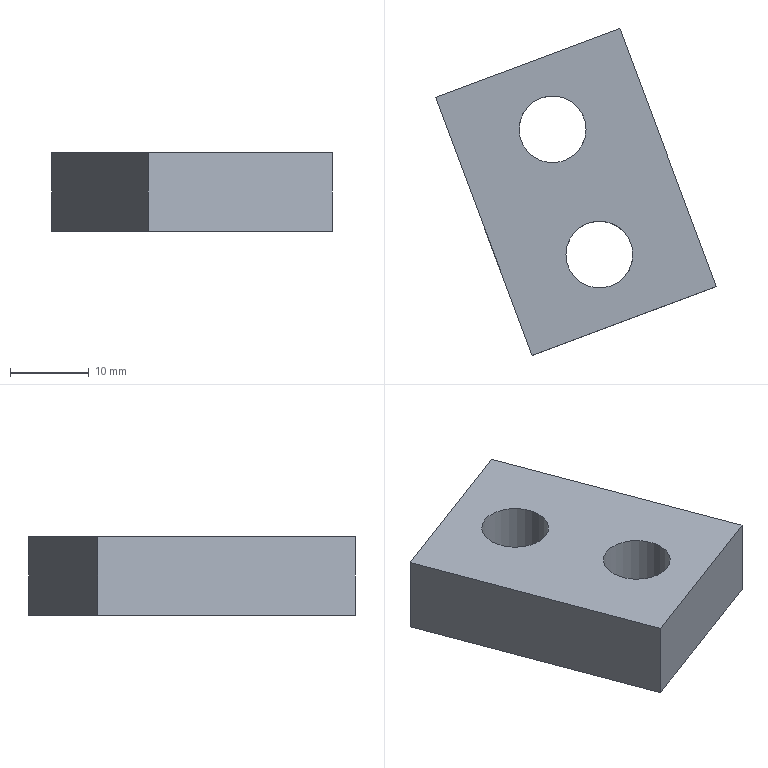Part | NX | features solid 2 | 1 solid | 8 faces | box 35.674 x 41.539 x 10 mm | volume 7615 mm3 | plane 6 | cylinder 2 | commonest cylinder face diameters 8.5 x2
STEP:
#1=CARTESIAN_POINT('',(89.721,-94.859,60.));
#2=VERTEX_POINT('',#1);
#3=CARTESIAN_POINT('',(89.721,-94.859,70.));
#4=VERTEX_POINT('',#3);
#5=CARTESIAN_POINT('',(89.721,-94.859,60.));
#6=DIRECTION('',(0.,0.,1.));
#7=VECTOR('',#6,1000.);
#8=LINE('',#5,#7);
#9=EDGE_CURVE('',#2,#4,#8,.T.);
#10=ORIENTED_EDGE('',*,*,#9,.T.);
#11=CARTESIAN_POINT('',(77.464,-62.075,70.));
#12=VERTEX_POINT('',#11);
#13=CARTESIAN_POINT('',(84.468,-80.808,70.));
#14=DIRECTION('',(-0.3502,0.9367,0.));
#15=VECTOR('',#14,1000.);
#16=LINE('',#13,#15);
#17=EDGE_CURVE('',#4,#12,#16,.T.);
#18=ORIENTED_EDGE('',*,*,#17,.T.);
#19=CARTESIAN_POINT('',(77.464,-62.075,60.));
#20=VERTEX_POINT('',#19);
#21=CARTESIAN_POINT('',(77.464,-62.075,60.));
#22=DIRECTION('',(0.,0.,1.));
#23=VECTOR('',#22,1000.);
#24=LINE('',#21,#23);
#25=EDGE_CURVE('',#20,#12,#24,.T.);
#26=ORIENTED_EDGE('',*,*,#25,.F.);
#27=CARTESIAN_POINT('',(84.468,-80.808,60.));
#28=DIRECTION('',(0.3502,-0.9367,0.));
#29=VECTOR('',#28,1000.);
#30=LINE('',#27,#29);
#31=EDGE_CURVE('',#20,#2,#30,.T.);
#32=ORIENTED_EDGE('',*,*,#31,.T.);
#33=EDGE_LOOP('',(#10,#18,#26,#32));
#34=FACE_BOUND('',#33,.T.);
#35=CARTESIAN_POINT('',(84.468,-80.808,60.));
#36=DIRECTION('',(-0.9367,-0.3502,0.));
#37=DIRECTION('',(0.,0.,1.));
#38=AXIS2_PLACEMENT_3D('',#35,#36,#37);
#39=PLANE('',#38);
#40=ADVANCED_FACE('',(#34),#39,.T.);
#41=CARTESIAN_POINT('',(102.527,-82.051,70.));
#42=VERTEX_POINT('',#41);
#43=CARTESIAN_POINT('',(98.277,-82.051,70.));
#44=DIRECTION('',(0.,0.,-1.));
#45=DIRECTION('',(1.,0.,0.));
#46=AXIS2_PLACEMENT_3D('',#43,#44,#45);
#47=CIRCLE('',#46,4.25);
#48=EDGE_CURVE('',#42,#42,#47,.T.);
#49=ORIENTED_EDGE('',*,*,#48,.F.);
#50=EDGE_LOOP('',(#49));
#51=FACE_BOUND('',#50,.T.);
#52=CARTESIAN_POINT('',(96.789,-78.07,60.));
#53=VERTEX_POINT('',#52);
#54=CARTESIAN_POINT('',(98.277,-82.051,60.));
#55=DIRECTION('',(0.,0.,1.));
#56=DIRECTION('',(-0.3502,0.9367,0.));
#57=AXIS2_PLACEMENT_3D('',#54,#55,#56);
#58=CIRCLE('',#57,4.25);
#59=EDGE_CURVE('',#53,#53,#58,.T.);
#60=ORIENTED_EDGE('',*,*,#59,.F.);
#61=EDGE_LOOP('',(#60));
#62=FACE_BOUND('',#61,.T.);
#63=CARTESIAN_POINT('',(98.277,-82.051,67.));
#64=DIRECTION('',(0.,0.,-1.));
#65=DIRECTION('',(0.3502,-0.9367,0.));
#66=AXIS2_PLACEMENT_3D('',#63,#64,#65);
#67=CYLINDRICAL_SURFACE('',#66,4.25);
#68=ADVANCED_FACE('',(#51,#62),#67,.F.);
#69=CARTESIAN_POINT('',(100.881,-53.32,60.));
#70=VERTEX_POINT('',#69);
#71=CARTESIAN_POINT('',(100.881,-53.32,70.));
#72=VERTEX_POINT('',#71);
#73=CARTESIAN_POINT('',(100.881,-53.32,60.));
#74=DIRECTION('',(0.,0.,1.));
#75=VECTOR('',#74,1000.);
#76=LINE('',#73,#75);
#77=EDGE_CURVE('',#70,#72,#76,.T.);
#78=ORIENTED_EDGE('',*,*,#77,.T.);
#79=CARTESIAN_POINT('',(113.138,-86.103,70.));
#80=VERTEX_POINT('',#79);
#81=CARTESIAN_POINT('',(107.885,-72.053,70.));
#82=DIRECTION('',(0.3502,-0.9367,0.));
#83=VECTOR('',#82,1000.);
#84=LINE('',#81,#83);
#85=EDGE_CURVE('',#72,#80,#84,.T.);
#86=ORIENTED_EDGE('',*,*,#85,.T.);
#87=CARTESIAN_POINT('',(113.138,-86.103,60.));
#88=VERTEX_POINT('',#87);
#89=CARTESIAN_POINT('',(113.138,-86.103,60.));
#90=DIRECTION('',(0.,0.,1.));
#91=VECTOR('',#90,1000.);
#92=LINE('',#89,#91);
#93=EDGE_CURVE('',#88,#80,#92,.T.);
#94=ORIENTED_EDGE('',*,*,#93,.F.);
#95=CARTESIAN_POINT('',(107.885,-72.053,60.));
#96=DIRECTION('',(-0.3502,0.9367,0.));
#97=VECTOR('',#96,1000.);
#98=LINE('',#95,#97);
#99=EDGE_CURVE('',#88,#70,#98,.T.);
#100=ORIENTED_EDGE('',*,*,#99,.T.);
#101=EDGE_LOOP('',(#78,#86,#94,#100));
#102=FACE_BOUND('',#101,.T.);
#103=CARTESIAN_POINT('',(107.885,-72.053,60.));
#104=DIRECTION('',(0.9367,0.3502,0.));
#105=DIRECTION('',(0.,0.,-1.));
#106=AXIS2_PLACEMENT_3D('',#103,#104,#105);
#107=PLANE('',#106);
#108=ADVANCED_FACE('',(#102),#107,.T.);
#109=ORIENTED_EDGE('',*,*,#25,.T.);
#110=CARTESIAN_POINT('',(89.172,-57.697,70.));
#111=DIRECTION('',(0.9367,0.3502,0.));
#112=VECTOR('',#111,1000.);
#113=LINE('',#110,#112);
#114=EDGE_CURVE('',#12,#72,#113,.T.);
#115=ORIENTED_EDGE('',*,*,#114,.T.);
#116=ORIENTED_EDGE('',*,*,#77,.F.);
#117=CARTESIAN_POINT('',(89.172,-57.697,60.));
#118=DIRECTION('',(-0.9367,-0.3502,0.));
#119=VECTOR('',#118,1000.);
#120=LINE('',#117,#119);
#121=EDGE_CURVE('',#70,#20,#120,.T.);
#122=ORIENTED_EDGE('',*,*,#121,.T.);
#123=EDGE_LOOP('',(#109,#115,#116,#122));
#124=FACE_BOUND('',#123,.T.);
#125=CARTESIAN_POINT('',(89.172,-57.697,60.));
#126=DIRECTION('',(-0.3502,0.9367,0.));
#127=DIRECTION('',(0.,0.,-1.));
#128=AXIS2_PLACEMENT_3D('',#125,#126,#127);
#129=PLANE('',#128);
#130=ADVANCED_FACE('',(#124),#129,.T.);
#131=CARTESIAN_POINT('',(101.429,-90.481,60.));
#132=DIRECTION('',(0.9367,0.3502,0.));
#133=VECTOR('',#132,1000.);
#134=LINE('',#131,#133);
#135=EDGE_CURVE('',#2,#88,#134,.T.);
#136=ORIENTED_EDGE('',*,*,#135,.T.);
#137=ORIENTED_EDGE('',*,*,#93,.T.);
#138=CARTESIAN_POINT('',(101.429,-90.481,70.));
#139=DIRECTION('',(-0.9367,-0.3502,0.));
#140=VECTOR('',#139,1000.);
#141=LINE('',#138,#140);
#142=EDGE_CURVE('',#80,#4,#141,.T.);
#143=ORIENTED_EDGE('',*,*,#142,.T.);
#144=ORIENTED_EDGE('',*,*,#9,.F.);
#145=EDGE_LOOP('',(#136,#137,#143,#144));
#146=FACE_BOUND('',#145,.T.);
#147=CARTESIAN_POINT('',(101.429,-90.481,60.));
#148=DIRECTION('',(0.3502,-0.9367,0.));
#149=DIRECTION('',(0.,0.,1.));
#150=AXIS2_PLACEMENT_3D('',#147,#148,#149);
#151=PLANE('',#150);
#152=ADVANCED_FACE('',(#146),#151,.T.);
#153=CARTESIAN_POINT('',(96.574,-66.127,70.));
#154=VERTEX_POINT('',#153);
#155=CARTESIAN_POINT('',(92.324,-66.127,70.));
#156=DIRECTION('',(0.,0.,-1.));
#157=DIRECTION('',(1.,0.,0.));
#158=AXIS2_PLACEMENT_3D('',#155,#156,#157);
#159=CIRCLE('',#158,4.25);
#160=EDGE_CURVE('',#154,#154,#159,.T.);
#161=ORIENTED_EDGE('',*,*,#160,.F.);
#162=EDGE_LOOP('',(#161));
#163=FACE_BOUND('',#162,.T.);
#164=CARTESIAN_POINT('',(90.836,-62.147,60.));
#165=VERTEX_POINT('',#164);
#166=CARTESIAN_POINT('',(92.324,-66.127,60.));
#167=DIRECTION('',(0.,0.,1.));
#168=DIRECTION('',(-0.3502,0.9367,0.));
#169=AXIS2_PLACEMENT_3D('',#166,#167,#168);
#170=CIRCLE('',#169,4.25);
#171=EDGE_CURVE('',#165,#165,#170,.T.);
#172=ORIENTED_EDGE('',*,*,#171,.F.);
#173=EDGE_LOOP('',(#172));
#174=FACE_BOUND('',#173,.T.);
#175=CARTESIAN_POINT('',(92.324,-66.127,67.));
#176=DIRECTION('',(0.,0.,-1.));
#177=DIRECTION('',(0.3502,-0.9367,0.));
#178=AXIS2_PLACEMENT_3D('',#175,#176,#177);
#179=CYLINDRICAL_SURFACE('',#178,4.25);
#180=ADVANCED_FACE('',(#163,#174),#179,.F.);
#181=ORIENTED_EDGE('',*,*,#171,.T.);
#182=EDGE_LOOP('',(#181));
#183=FACE_BOUND('',#182,.T.);
#184=ORIENTED_EDGE('',*,*,#135,.F.);
#185=ORIENTED_EDGE('',*,*,#31,.F.);
#186=ORIENTED_EDGE('',*,*,#121,.F.);
#187=ORIENTED_EDGE('',*,*,#99,.F.);
#188=EDGE_LOOP('',(#184,#185,#186,#187));
#189=FACE_BOUND('',#188,.T.);
#190=ORIENTED_EDGE('',*,*,#59,.T.);
#191=EDGE_LOOP('',(#190));
#192=FACE_BOUND('',#191,.T.);
#193=CARTESIAN_POINT('',(96.176,-76.431,60.));
#194=DIRECTION('',(0.,0.,-1.));
#195=DIRECTION('',(0.3502,-0.9367,0.));
#196=AXIS2_PLACEMENT_3D('',#193,#194,#195);
#197=PLANE('',#196);
#198=ADVANCED_FACE('',(#183,#189,#192),#197,.T.);
#199=ORIENTED_EDGE('',*,*,#160,.T.);
#200=EDGE_LOOP('',(#199));
#201=FACE_BOUND('',#200,.T.);
#202=ORIENTED_EDGE('',*,*,#17,.F.);
#203=ORIENTED_EDGE('',*,*,#142,.F.);
#204=ORIENTED_EDGE('',*,*,#85,.F.);
#205=ORIENTED_EDGE('',*,*,#114,.F.);
#206=EDGE_LOOP('',(#202,#203,#204,#205));
#207=FACE_BOUND('',#206,.T.);
#208=ORIENTED_EDGE('',*,*,#48,.T.);
#209=EDGE_LOOP('',(#208));
#210=FACE_BOUND('',#209,.T.);
#211=CARTESIAN_POINT('',(96.176,-76.431,70.));
#212=DIRECTION('',(0.,0.,1.));
#213=DIRECTION('',(-0.3502,0.9367,0.));
#214=AXIS2_PLACEMENT_3D('',#211,#212,#213);
#215=PLANE('',#214);
#216=ADVANCED_FACE('',(#201,#207,#210),#215,.T.);
#217=CLOSED_SHELL('',(#40,#68,#108,#130,#152,#180,#198,#216));
#218=MANIFOLD_SOLID_BREP('',#217);
#219=(LENGTH_UNIT()NAMED_UNIT(*)SI_UNIT(.MILLI.,.METRE.));
#220=UNCERTAINTY_MEASURE_WITH_UNIT(LENGTH_MEASURE(0.00001),#219,'','');
#221=(NAMED_UNIT(*)PLANE_ANGLE_UNIT()SI_UNIT($,.RADIAN.));
#222=(NAMED_UNIT(*)SI_UNIT($,.STERADIAN.)SOLID_ANGLE_UNIT());
#223=(GEOMETRIC_REPRESENTATION_CONTEXT(3)GLOBAL_UNCERTAINTY_ASSIGNED_CONTEXT((#220))GLOBAL_UNIT_ASSIGNED_CONTEXT((#219,#221,#222))REPRESENTATION_CONTEXT('',''));
#224=ADVANCED_BREP_SHAPE_REPRESENTATION('',(#218),#223);